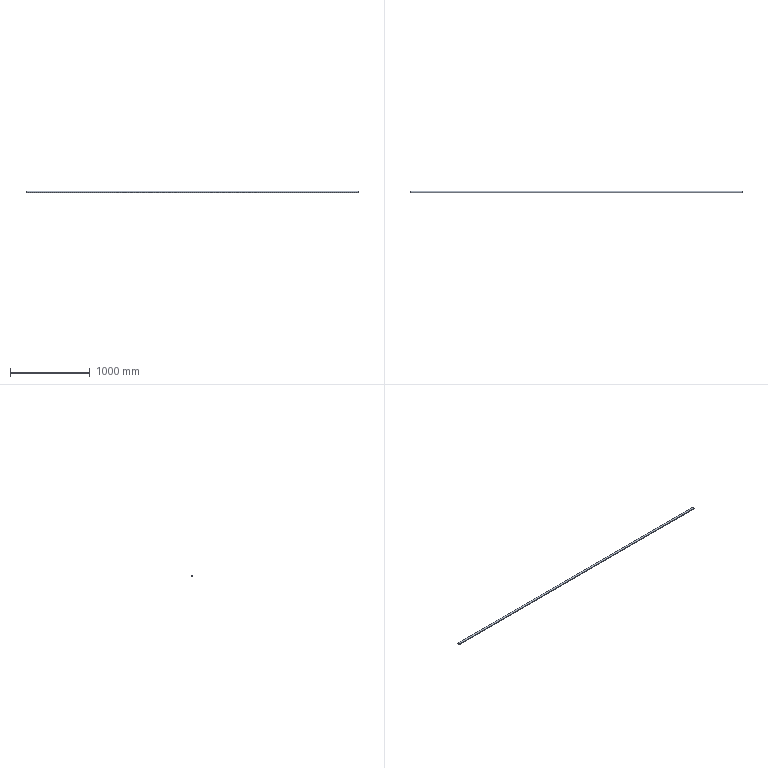Part | STEP file | E3-粉仓护栏栏杆8_Default<As Machined> | 1 solid | 6 faces | box 4175 x 25 x 25 mm | volume 462344 mm3 | cylinder 4 | plane 2 | commonest cylinder face diameters 22 x2 25 x2
STEP:
#1=CARTESIAN_POINT('',(0.,0.,0.));
#2=DIRECTION('',(0.,0.,1.));
#3=DIRECTION('',(1.,0.,0.));
#4=AXIS2_PLACEMENT_3D('',#1,#2,#3);
#5=CARTESIAN_POINT('',(2087.5,-12.5,0.));
#6=VERTEX_POINT('',#5);
#7=CARTESIAN_POINT('',(2087.5,12.5,0.));
#8=VERTEX_POINT('',#7);
#9=CARTESIAN_POINT('',(2087.5,0.,0.));
#10=DIRECTION('',(-1.,0.,0.));
#11=DIRECTION('',(0.,1.,0.));
#12=AXIS2_PLACEMENT_3D('',#9,#10,#11);
#13=CIRCLE('',#12,12.5);
#14=CARTESIAN_POINT('',(2087.5,0.,0.));
#15=DIRECTION('',(-1.,0.,0.));
#16=DIRECTION('',(0.,-1.,0.));
#17=AXIS2_PLACEMENT_3D('',#14,#15,#16);
#18=CYLINDRICAL_SURFACE('',#17,12.5);
#19=CARTESIAN_POINT('',(-3.142,0.));
#20=DIRECTION('',(1.,0.));
#21=VECTOR('',#20,1.);
#22=LINE('',#19,#21);
#23=(GEOMETRIC_REPRESENTATION_CONTEXT(2)PARAMETRIC_REPRESENTATION_CONTEXT()REPRESENTATION_CONTEXT('',''));
#24=DEFINITIONAL_REPRESENTATION('',(#22),#23);
#25=PCURVE('',#18,#24);
#26=CARTESIAN_POINT('',(2087.5,0.,0.));
#27=DIRECTION('',(1.,0.,0.));
#28=DIRECTION('',(0.,1.,0.));
#29=AXIS2_PLACEMENT_3D('',#26,#27,#28);
#30=PLANE('',#29);
#31=CARTESIAN_POINT('',(12.5,0.));
#32=CARTESIAN_POINT('',(12.5,-21.651));
#33=CARTESIAN_POINT('',(-6.25,-10.825));
#34=CARTESIAN_POINT('',(-25.,0.));
#35=CARTESIAN_POINT('',(-6.25,10.825));
#36=CARTESIAN_POINT('',(12.5,21.651));
#37=CARTESIAN_POINT('',(12.5,0.));
#38=(BOUNDED_CURVE()B_SPLINE_CURVE(2,(#31,#32,#33,#34,#35,#36,#37),.UNSPECIFIED.,.T.,.F.)B_SPLINE_CURVE_WITH_KNOTS((1,2,2,2,2,1),(-2.094,0.,2.094,4.189,6.283,8.378),.UNSPECIFIED.)CURVE()GEOMETRIC_REPRESENTATION_ITEM()RATIONAL_B_SPLINE_CURVE((1.,0.5,1.,0.5,1.,0.5,1.))REPRESENTATION_ITEM(''));
#39=(GEOMETRIC_REPRESENTATION_CONTEXT(2)PARAMETRIC_REPRESENTATION_CONTEXT()REPRESENTATION_CONTEXT('',''));
#40=DEFINITIONAL_REPRESENTATION('',(#38),#39);
#41=PCURVE('',#30,#40);
#42=SURFACE_CURVE('',#13,(#25,#41),.PCURVE_S1.);
#43=EDGE_CURVE('',#6,#8,#42,.T.);
#44=ORIENTED_EDGE('',*,*,#43,.T.);
#45=CARTESIAN_POINT('',(-2087.5,12.5,0.));
#46=VERTEX_POINT('',#45);
#47=CARTESIAN_POINT('',(2087.5,12.5,0.));
#48=DIRECTION('',(-1.,0.,0.));
#49=VECTOR('',#48,1.);
#50=LINE('',#47,#49);
#51=CARTESIAN_POINT('',(3.142,0.));
#52=DIRECTION('',(0.,1.));
#53=VECTOR('',#52,1.);
#54=LINE('',#51,#53);
#55=(GEOMETRIC_REPRESENTATION_CONTEXT(2)PARAMETRIC_REPRESENTATION_CONTEXT()REPRESENTATION_CONTEXT('',''));
#56=DEFINITIONAL_REPRESENTATION('',(#54),#55);
#57=PCURVE('',#18,#56);
#58=CARTESIAN_POINT('',(2087.5,0.,0.));
#59=DIRECTION('',(-1.,0.,0.));
#60=DIRECTION('',(0.,-1.,0.));
#61=AXIS2_PLACEMENT_3D('',#58,#59,#60);
#62=CYLINDRICAL_SURFACE('',#61,12.5);
#63=CARTESIAN_POINT('',(3.142,0.));
#64=DIRECTION('',(0.,1.));
#65=VECTOR('',#64,1.);
#66=LINE('',#63,#65);
#67=(GEOMETRIC_REPRESENTATION_CONTEXT(2)PARAMETRIC_REPRESENTATION_CONTEXT()REPRESENTATION_CONTEXT('',''));
#68=DEFINITIONAL_REPRESENTATION('',(#66),#67);
#69=PCURVE('',#62,#68);
#70=SURFACE_CURVE('',#50,(#57,#69),.PCURVE_S1.);
#71=EDGE_CURVE('',#8,#46,#70,.T.);
#72=ORIENTED_EDGE('',*,*,#71,.T.);
#73=CARTESIAN_POINT('',(-2087.5,-12.5,0.));
#74=VERTEX_POINT('',#73);
#75=CARTESIAN_POINT('',(-2087.5,0.,0.));
#76=DIRECTION('',(-1.,0.,0.));
#77=DIRECTION('',(0.,1.,0.));
#78=AXIS2_PLACEMENT_3D('',#75,#76,#77);
#79=CIRCLE('',#78,12.5);
#80=CARTESIAN_POINT('',(-3.142,4175.));
#81=DIRECTION('',(1.,0.));
#82=VECTOR('',#81,1.);
#83=LINE('',#80,#82);
#84=(GEOMETRIC_REPRESENTATION_CONTEXT(2)PARAMETRIC_REPRESENTATION_CONTEXT()REPRESENTATION_CONTEXT('',''));
#85=DEFINITIONAL_REPRESENTATION('',(#83),#84);
#86=PCURVE('',#18,#85);
#87=CARTESIAN_POINT('',(-2087.5,0.,0.));
#88=DIRECTION('',(1.,0.,0.));
#89=DIRECTION('',(0.,1.,0.));
#90=AXIS2_PLACEMENT_3D('',#87,#88,#89);
#91=PLANE('',#90);
#92=CARTESIAN_POINT('',(12.5,0.));
#93=CARTESIAN_POINT('',(12.5,-21.651));
#94=CARTESIAN_POINT('',(-6.25,-10.825));
#95=CARTESIAN_POINT('',(-25.,0.));
#96=CARTESIAN_POINT('',(-6.25,10.825));
#97=CARTESIAN_POINT('',(12.5,21.651));
#98=CARTESIAN_POINT('',(12.5,0.));
#99=(BOUNDED_CURVE()B_SPLINE_CURVE(2,(#92,#93,#94,#95,#96,#97,#98),.UNSPECIFIED.,.T.,.F.)B_SPLINE_CURVE_WITH_KNOTS((1,2,2,2,2,1),(-2.094,0.,2.094,4.189,6.283,8.378),.UNSPECIFIED.)CURVE()GEOMETRIC_REPRESENTATION_ITEM()RATIONAL_B_SPLINE_CURVE((1.,0.5,1.,0.5,1.,0.5,1.))REPRESENTATION_ITEM(''));
#100=(GEOMETRIC_REPRESENTATION_CONTEXT(2)PARAMETRIC_REPRESENTATION_CONTEXT()REPRESENTATION_CONTEXT('',''));
#101=DEFINITIONAL_REPRESENTATION('',(#99),#100);
#102=PCURVE('',#91,#101);
#103=SURFACE_CURVE('',#79,(#86,#102),.PCURVE_S1.);
#104=EDGE_CURVE('',#74,#46,#103,.T.);
#105=ORIENTED_EDGE('',*,*,#104,.F.);
#106=CARTESIAN_POINT('',(2087.5,-12.5,0.));
#107=DIRECTION('',(-1.,0.,0.));
#108=VECTOR('',#107,1.);
#109=LINE('',#106,#108);
#110=CARTESIAN_POINT('',(0.,0.));
#111=DIRECTION('',(0.,1.));
#112=VECTOR('',#111,1.);
#113=LINE('',#110,#112);
#114=(GEOMETRIC_REPRESENTATION_CONTEXT(2)PARAMETRIC_REPRESENTATION_CONTEXT()REPRESENTATION_CONTEXT('',''));
#115=DEFINITIONAL_REPRESENTATION('',(#113),#114);
#116=PCURVE('',#18,#115);
#117=CARTESIAN_POINT('',(6.283,0.));
#118=DIRECTION('',(0.,1.));
#119=VECTOR('',#118,1.);
#120=LINE('',#117,#119);
#121=(GEOMETRIC_REPRESENTATION_CONTEXT(2)PARAMETRIC_REPRESENTATION_CONTEXT()REPRESENTATION_CONTEXT('',''));
#122=DEFINITIONAL_REPRESENTATION('',(#120),#121);
#123=PCURVE('',#62,#122);
#124=SURFACE_CURVE('',#109,(#116,#123),.PCURVE_S1.);
#125=EDGE_CURVE('',#6,#74,#124,.T.);
#126=ORIENTED_EDGE('',*,*,#125,.F.);
#127=EDGE_LOOP('',(#44,#72,#105,#126));
#128=FACE_BOUND('',#127,.T.);
#129=ADVANCED_FACE('',(#128),#18,.T.);
#130=CARTESIAN_POINT('',(2087.5,-11.,0.));
#131=VERTEX_POINT('',#130);
#132=CARTESIAN_POINT('',(-2087.5,-11.,0.));
#133=VERTEX_POINT('',#132);
#134=CARTESIAN_POINT('',(2087.5,-11.,0.));
#135=DIRECTION('',(-1.,0.,0.));
#136=VECTOR('',#135,1.);
#137=LINE('',#134,#136);
#138=CARTESIAN_POINT('',(2087.5,0.,0.));
#139=DIRECTION('',(-1.,0.,0.));
#140=DIRECTION('',(0.,-1.,0.));
#141=AXIS2_PLACEMENT_3D('',#138,#139,#140);
#142=CYLINDRICAL_SURFACE('',#141,11.);
#143=CARTESIAN_POINT('',(6.283,0.));
#144=DIRECTION('',(0.,1.));
#145=VECTOR('',#144,1.);
#146=LINE('',#143,#145);
#147=(GEOMETRIC_REPRESENTATION_CONTEXT(2)PARAMETRIC_REPRESENTATION_CONTEXT()REPRESENTATION_CONTEXT('',''));
#148=DEFINITIONAL_REPRESENTATION('',(#146),#147);
#149=PCURVE('',#142,#148);
#150=CARTESIAN_POINT('',(2087.5,0.,0.));
#151=DIRECTION('',(-1.,0.,0.));
#152=DIRECTION('',(0.,-1.,0.));
#153=AXIS2_PLACEMENT_3D('',#150,#151,#152);
#154=CYLINDRICAL_SURFACE('',#153,11.);
#155=CARTESIAN_POINT('',(0.,0.));
#156=DIRECTION('',(0.,1.));
#157=VECTOR('',#156,1.);
#158=LINE('',#155,#157);
#159=(GEOMETRIC_REPRESENTATION_CONTEXT(2)PARAMETRIC_REPRESENTATION_CONTEXT()REPRESENTATION_CONTEXT('',''));
#160=DEFINITIONAL_REPRESENTATION('',(#158),#159);
#161=PCURVE('',#154,#160);
#162=SURFACE_CURVE('',#137,(#149,#161),.PCURVE_S1.);
#163=EDGE_CURVE('',#131,#133,#162,.T.);
#164=ORIENTED_EDGE('',*,*,#163,.T.);
#165=CARTESIAN_POINT('',(-2087.5,11.,0.));
#166=VERTEX_POINT('',#165);
#167=CARTESIAN_POINT('',(-2087.5,0.,0.));
#168=DIRECTION('',(-1.,0.,0.));
#169=DIRECTION('',(0.,1.,0.));
#170=AXIS2_PLACEMENT_3D('',#167,#168,#169);
#171=CIRCLE('',#170,11.);
#172=CARTESIAN_POINT('',(3.142,4175.));
#173=DIRECTION('',(1.,0.));
#174=VECTOR('',#173,1.);
#175=LINE('',#172,#174);
#176=(GEOMETRIC_REPRESENTATION_CONTEXT(2)PARAMETRIC_REPRESENTATION_CONTEXT()REPRESENTATION_CONTEXT('',''));
#177=DEFINITIONAL_REPRESENTATION('',(#175),#176);
#178=PCURVE('',#142,#177);
#179=CARTESIAN_POINT('',(11.,0.));
#180=CARTESIAN_POINT('',(11.,-19.053));
#181=CARTESIAN_POINT('',(-5.5,-9.526));
#182=CARTESIAN_POINT('',(-22.,0.));
#183=CARTESIAN_POINT('',(-5.5,9.526));
#184=CARTESIAN_POINT('',(11.,19.053));
#185=CARTESIAN_POINT('',(11.,0.));
#186=(BOUNDED_CURVE()B_SPLINE_CURVE(2,(#179,#180,#181,#182,#183,#184,#185),.UNSPECIFIED.,.T.,.F.)B_SPLINE_CURVE_WITH_KNOTS((1,2,2,2,2,1),(-2.094,0.,2.094,4.189,6.283,8.378),.UNSPECIFIED.)CURVE()GEOMETRIC_REPRESENTATION_ITEM()RATIONAL_B_SPLINE_CURVE((1.,0.5,1.,0.5,1.,0.5,1.))REPRESENTATION_ITEM(''));
#187=(GEOMETRIC_REPRESENTATION_CONTEXT(2)PARAMETRIC_REPRESENTATION_CONTEXT()REPRESENTATION_CONTEXT('',''));
#188=DEFINITIONAL_REPRESENTATION('',(#186),#187);
#189=PCURVE('',#91,#188);
#190=SURFACE_CURVE('',#171,(#178,#189),.PCURVE_S1.);
#191=EDGE_CURVE('',#166,#133,#190,.T.);
#192=ORIENTED_EDGE('',*,*,#191,.F.);
#193=CARTESIAN_POINT('',(2087.5,11.,0.));
#194=VERTEX_POINT('',#193);
#195=CARTESIAN_POINT('',(2087.5,11.,0.));
#196=DIRECTION('',(-1.,0.,0.));
#197=VECTOR('',#196,1.);
#198=LINE('',#195,#197);
#199=CARTESIAN_POINT('',(3.142,0.));
#200=DIRECTION('',(0.,1.));
#201=VECTOR('',#200,1.);
#202=LINE('',#199,#201);
#203=(GEOMETRIC_REPRESENTATION_CONTEXT(2)PARAMETRIC_REPRESENTATION_CONTEXT()REPRESENTATION_CONTEXT('',''));
#204=DEFINITIONAL_REPRESENTATION('',(#202),#203);
#205=PCURVE('',#142,#204);
#206=CARTESIAN_POINT('',(3.142,0.));
#207=DIRECTION('',(0.,1.));
#208=VECTOR('',#207,1.);
#209=LINE('',#206,#208);
#210=(GEOMETRIC_REPRESENTATION_CONTEXT(2)PARAMETRIC_REPRESENTATION_CONTEXT()REPRESENTATION_CONTEXT('',''));
#211=DEFINITIONAL_REPRESENTATION('',(#209),#210);
#212=PCURVE('',#154,#211);
#213=SURFACE_CURVE('',#198,(#205,#212),.PCURVE_S1.);
#214=EDGE_CURVE('',#194,#166,#213,.T.);
#215=ORIENTED_EDGE('',*,*,#214,.F.);
#216=CARTESIAN_POINT('',(2087.5,0.,0.));
#217=DIRECTION('',(-1.,0.,0.));
#218=DIRECTION('',(0.,1.,0.));
#219=AXIS2_PLACEMENT_3D('',#216,#217,#218);
#220=CIRCLE('',#219,11.);
#221=CARTESIAN_POINT('',(3.142,0.));
#222=DIRECTION('',(1.,0.));
#223=VECTOR('',#222,1.);
#224=LINE('',#221,#223);
#225=(GEOMETRIC_REPRESENTATION_CONTEXT(2)PARAMETRIC_REPRESENTATION_CONTEXT()REPRESENTATION_CONTEXT('',''));
#226=DEFINITIONAL_REPRESENTATION('',(#224),#225);
#227=PCURVE('',#142,#226);
#228=CARTESIAN_POINT('',(11.,0.));
#229=CARTESIAN_POINT('',(11.,-19.053));
#230=CARTESIAN_POINT('',(-5.5,-9.526));
#231=CARTESIAN_POINT('',(-22.,0.));
#232=CARTESIAN_POINT('',(-5.5,9.526));
#233=CARTESIAN_POINT('',(11.,19.053));
#234=CARTESIAN_POINT('',(11.,0.));
#235=(BOUNDED_CURVE()B_SPLINE_CURVE(2,(#228,#229,#230,#231,#232,#233,#234),.UNSPECIFIED.,.T.,.F.)B_SPLINE_CURVE_WITH_KNOTS((1,2,2,2,2,1),(-2.094,0.,2.094,4.189,6.283,8.378),.UNSPECIFIED.)CURVE()GEOMETRIC_REPRESENTATION_ITEM()RATIONAL_B_SPLINE_CURVE((1.,0.5,1.,0.5,1.,0.5,1.))REPRESENTATION_ITEM(''));
#236=(GEOMETRIC_REPRESENTATION_CONTEXT(2)PARAMETRIC_REPRESENTATION_CONTEXT()REPRESENTATION_CONTEXT('',''));
#237=DEFINITIONAL_REPRESENTATION('',(#235),#236);
#238=PCURVE('',#30,#237);
#239=SURFACE_CURVE('',#220,(#227,#238),.PCURVE_S1.);
#240=EDGE_CURVE('',#194,#131,#239,.T.);
#241=ORIENTED_EDGE('',*,*,#240,.T.);
#242=EDGE_LOOP('',(#164,#192,#215,#241));
#243=FACE_BOUND('',#242,.F.);
#244=ADVANCED_FACE('',(#243),#142,.F.);
#245=CARTESIAN_POINT('',(-2087.5,0.,0.));
#246=DIRECTION('',(-1.,0.,0.));
#247=DIRECTION('',(0.,1.,0.));
#248=AXIS2_PLACEMENT_3D('',#245,#246,#247);
#249=CIRCLE('',#248,11.);
#250=CARTESIAN_POINT('',(-3.142,4175.));
#251=DIRECTION('',(1.,0.));
#252=VECTOR('',#251,1.);
#253=LINE('',#250,#252);
#254=(GEOMETRIC_REPRESENTATION_CONTEXT(2)PARAMETRIC_REPRESENTATION_CONTEXT()REPRESENTATION_CONTEXT('',''));
#255=DEFINITIONAL_REPRESENTATION('',(#253),#254);
#256=PCURVE('',#154,#255);
#257=CARTESIAN_POINT('',(11.,0.));
#258=CARTESIAN_POINT('',(11.,-19.053));
#259=CARTESIAN_POINT('',(-5.5,-9.526));
#260=CARTESIAN_POINT('',(-22.,0.));
#261=CARTESIAN_POINT('',(-5.5,9.526));
#262=CARTESIAN_POINT('',(11.,19.053));
#263=CARTESIAN_POINT('',(11.,0.));
#264=(BOUNDED_CURVE()B_SPLINE_CURVE(2,(#257,#258,#259,#260,#261,#262,#263),.UNSPECIFIED.,.T.,.F.)B_SPLINE_CURVE_WITH_KNOTS((1,2,2,2,2,1),(-2.094,0.,2.094,4.189,6.283,8.378),.UNSPECIFIED.)CURVE()GEOMETRIC_REPRESENTATION_ITEM()RATIONAL_B_SPLINE_CURVE((1.,0.5,1.,0.5,1.,0.5,1.))REPRESENTATION_ITEM(''));
#265=(GEOMETRIC_REPRESENTATION_CONTEXT(2)PARAMETRIC_REPRESENTATION_CONTEXT()REPRESENTATION_CONTEXT('',''));
#266=DEFINITIONAL_REPRESENTATION('',(#264),#265);
#267=PCURVE('',#91,#266);
#268=SURFACE_CURVE('',#249,(#256,#267),.PCURVE_S1.);
#269=EDGE_CURVE('',#133,#166,#268,.T.);
#270=ORIENTED_EDGE('',*,*,#269,.F.);
#271=ORIENTED_EDGE('',*,*,#163,.F.);
#272=CARTESIAN_POINT('',(2087.5,0.,0.));
#273=DIRECTION('',(-1.,0.,0.));
#274=DIRECTION('',(0.,1.,0.));
#275=AXIS2_PLACEMENT_3D('',#272,#273,#274);
#276=CIRCLE('',#275,11.);
#277=CARTESIAN_POINT('',(-3.142,0.));
#278=DIRECTION('',(1.,0.));
#279=VECTOR('',#278,1.);
#280=LINE('',#277,#279);
#281=(GEOMETRIC_REPRESENTATION_CONTEXT(2)PARAMETRIC_REPRESENTATION_CONTEXT()REPRESENTATION_CONTEXT('',''));
#282=DEFINITIONAL_REPRESENTATION('',(#280),#281);
#283=PCURVE('',#154,#282);
#284=CARTESIAN_POINT('',(11.,0.));
#285=CARTESIAN_POINT('',(11.,-19.053));
#286=CARTESIAN_POINT('',(-5.5,-9.526));
#287=CARTESIAN_POINT('',(-22.,0.));
#288=CARTESIAN_POINT('',(-5.5,9.526));
#289=CARTESIAN_POINT('',(11.,19.053));
#290=CARTESIAN_POINT('',(11.,0.));
#291=(BOUNDED_CURVE()B_SPLINE_CURVE(2,(#284,#285,#286,#287,#288,#289,#290),.UNSPECIFIED.,.T.,.F.)B_SPLINE_CURVE_WITH_KNOTS((1,2,2,2,2,1),(-2.094,0.,2.094,4.189,6.283,8.378),.UNSPECIFIED.)CURVE()GEOMETRIC_REPRESENTATION_ITEM()RATIONAL_B_SPLINE_CURVE((1.,0.5,1.,0.5,1.,0.5,1.))REPRESENTATION_ITEM(''));
#292=(GEOMETRIC_REPRESENTATION_CONTEXT(2)PARAMETRIC_REPRESENTATION_CONTEXT()REPRESENTATION_CONTEXT('',''));
#293=DEFINITIONAL_REPRESENTATION('',(#291),#292);
#294=PCURVE('',#30,#293);
#295=SURFACE_CURVE('',#276,(#283,#294),.PCURVE_S1.);
#296=EDGE_CURVE('',#131,#194,#295,.T.);
#297=ORIENTED_EDGE('',*,*,#296,.T.);
#298=ORIENTED_EDGE('',*,*,#214,.T.);
#299=EDGE_LOOP('',(#270,#271,#297,#298));
#300=FACE_BOUND('',#299,.F.);
#301=ADVANCED_FACE('',(#300),#154,.F.);
#302=ORIENTED_EDGE('',*,*,#71,.F.);
#303=CARTESIAN_POINT('',(2087.5,0.,0.));
#304=DIRECTION('',(-1.,0.,0.));
#305=DIRECTION('',(0.,1.,0.));
#306=AXIS2_PLACEMENT_3D('',#303,#304,#305);
#307=CIRCLE('',#306,12.5);
#308=CARTESIAN_POINT('',(3.142,0.));
#309=DIRECTION('',(1.,0.));
#310=VECTOR('',#309,1.);
#311=LINE('',#308,#310);
#312=(GEOMETRIC_REPRESENTATION_CONTEXT(2)PARAMETRIC_REPRESENTATION_CONTEXT()REPRESENTATION_CONTEXT('',''));
#313=DEFINITIONAL_REPRESENTATION('',(#311),#312);
#314=PCURVE('',#62,#313);
#315=CARTESIAN_POINT('',(12.5,0.));
#316=CARTESIAN_POINT('',(12.5,-21.651));
#317=CARTESIAN_POINT('',(-6.25,-10.825));
#318=CARTESIAN_POINT('',(-25.,0.));
#319=CARTESIAN_POINT('',(-6.25,10.825));
#320=CARTESIAN_POINT('',(12.5,21.651));
#321=CARTESIAN_POINT('',(12.5,0.));
#322=(BOUNDED_CURVE()B_SPLINE_CURVE(2,(#315,#316,#317,#318,#319,#320,#321),.UNSPECIFIED.,.T.,.F.)B_SPLINE_CURVE_WITH_KNOTS((1,2,2,2,2,1),(-2.094,0.,2.094,4.189,6.283,8.378),.UNSPECIFIED.)CURVE()GEOMETRIC_REPRESENTATION_ITEM()RATIONAL_B_SPLINE_CURVE((1.,0.5,1.,0.5,1.,0.5,1.))REPRESENTATION_ITEM(''));
#323=(GEOMETRIC_REPRESENTATION_CONTEXT(2)PARAMETRIC_REPRESENTATION_CONTEXT()REPRESENTATION_CONTEXT('',''));
#324=DEFINITIONAL_REPRESENTATION('',(#322),#323);
#325=PCURVE('',#30,#324);
#326=SURFACE_CURVE('',#307,(#314,#325),.PCURVE_S1.);
#327=EDGE_CURVE('',#8,#6,#326,.T.);
#328=ORIENTED_EDGE('',*,*,#327,.T.);
#329=ORIENTED_EDGE('',*,*,#125,.T.);
#330=CARTESIAN_POINT('',(-2087.5,0.,0.));
#331=DIRECTION('',(-1.,0.,0.));
#332=DIRECTION('',(0.,1.,0.));
#333=AXIS2_PLACEMENT_3D('',#330,#331,#332);
#334=CIRCLE('',#333,12.5);
#335=CARTESIAN_POINT('',(3.142,4175.));
#336=DIRECTION('',(1.,0.));
#337=VECTOR('',#336,1.);
#338=LINE('',#335,#337);
#339=(GEOMETRIC_REPRESENTATION_CONTEXT(2)PARAMETRIC_REPRESENTATION_CONTEXT()REPRESENTATION_CONTEXT('',''));
#340=DEFINITIONAL_REPRESENTATION('',(#338),#339);
#341=PCURVE('',#62,#340);
#342=CARTESIAN_POINT('',(12.5,0.));
#343=CARTESIAN_POINT('',(12.5,-21.651));
#344=CARTESIAN_POINT('',(-6.25,-10.825));
#345=CARTESIAN_POINT('',(-25.,0.));
#346=CARTESIAN_POINT('',(-6.25,10.825));
#347=CARTESIAN_POINT('',(12.5,21.651));
#348=CARTESIAN_POINT('',(12.5,0.));
#349=(BOUNDED_CURVE()B_SPLINE_CURVE(2,(#342,#343,#344,#345,#346,#347,#348),.UNSPECIFIED.,.T.,.F.)B_SPLINE_CURVE_WITH_KNOTS((1,2,2,2,2,1),(-2.094,0.,2.094,4.189,6.283,8.378),.UNSPECIFIED.)CURVE()GEOMETRIC_REPRESENTATION_ITEM()RATIONAL_B_SPLINE_CURVE((1.,0.5,1.,0.5,1.,0.5,1.))REPRESENTATION_ITEM(''));
#350=(GEOMETRIC_REPRESENTATION_CONTEXT(2)PARAMETRIC_REPRESENTATION_CONTEXT()REPRESENTATION_CONTEXT('',''));
#351=DEFINITIONAL_REPRESENTATION('',(#349),#350);
#352=PCURVE('',#91,#351);
#353=SURFACE_CURVE('',#334,(#341,#352),.PCURVE_S1.);
#354=EDGE_CURVE('',#46,#74,#353,.T.);
#355=ORIENTED_EDGE('',*,*,#354,.F.);
#356=EDGE_LOOP('',(#302,#328,#329,#355));
#357=FACE_BOUND('',#356,.T.);
#358=ADVANCED_FACE('',(#357),#62,.T.);
#359=ORIENTED_EDGE('',*,*,#296,.T.);
#360=ORIENTED_EDGE('',*,*,#240,.T.);
#361=EDGE_LOOP('',(#359,#360));
#362=FACE_BOUND('',#361,.T.);
#363=ORIENTED_EDGE('',*,*,#43,.F.);
#364=ORIENTED_EDGE('',*,*,#327,.F.);
#365=EDGE_LOOP('',(#363,#364));
#366=FACE_BOUND('',#365,.T.);
#367=ADVANCED_FACE('',(#362,#366),#30,.T.);
#368=ORIENTED_EDGE('',*,*,#269,.F.);
#369=ORIENTED_EDGE('',*,*,#191,.F.);
#370=EDGE_LOOP('',(#368,#369));
#371=FACE_BOUND('',#370,.T.);
#372=ORIENTED_EDGE('',*,*,#104,.T.);
#373=ORIENTED_EDGE('',*,*,#354,.T.);
#374=EDGE_LOOP('',(#372,#373));
#375=FACE_BOUND('',#374,.T.);
#376=ADVANCED_FACE('',(#371,#375),#91,.F.);
#377=CLOSED_SHELL('',(#129,#244,#301,#358,#367,#376));
#378=MANIFOLD_SOLID_BREP('',#377);
#379=(LENGTH_UNIT()NAMED_UNIT(*)SI_UNIT(.MILLI.,.METRE.));
#380=UNCERTAINTY_MEASURE_WITH_UNIT(LENGTH_MEASURE(0.0000001),#379,'','');
#381=(NAMED_UNIT(*)PLANE_ANGLE_UNIT()SI_UNIT($,.RADIAN.));
#382=(NAMED_UNIT(*)SI_UNIT($,.STERADIAN.)SOLID_ANGLE_UNIT());
#383=(GEOMETRIC_REPRESENTATION_CONTEXT(3)GLOBAL_UNCERTAINTY_ASSIGNED_CONTEXT((#380))GLOBAL_UNIT_ASSIGNED_CONTEXT((#379,#381,#382))REPRESENTATION_CONTEXT('',''));
#384=ADVANCED_BREP_SHAPE_REPRESENTATION('',(#4,#378),#383);